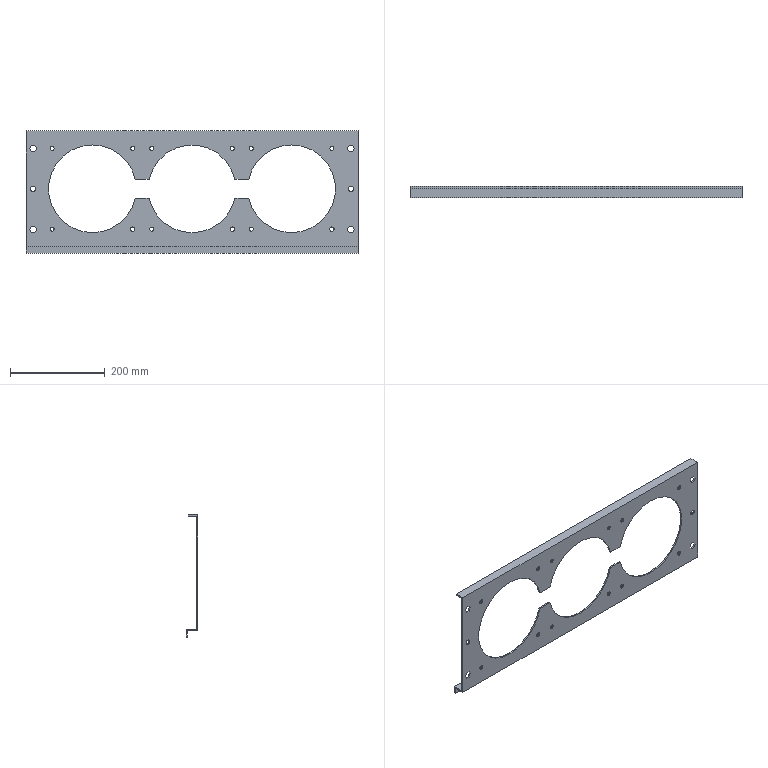Part | SolidWorks | features BaseBody 1 | 1 solid | 77 faces | box 700 x 25 x 258 mm | volume 370985 mm3 | plane 40 | cylinder 37 | commonest cylinder face diameters 8.5 x18 185 x9 9.1 x6 11 x4